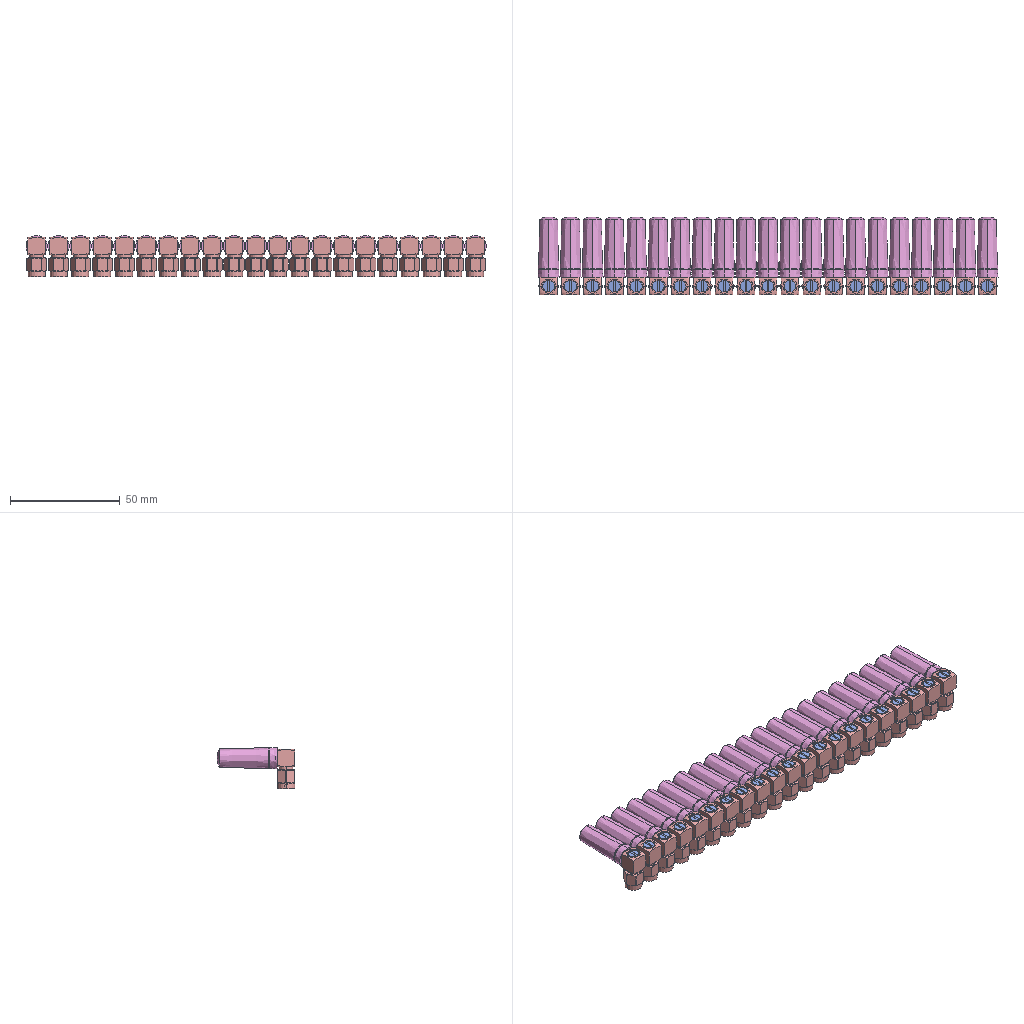Assembly | SolidWorks | 5 different items | 105 placed | box 210 x 36 x 19 mm
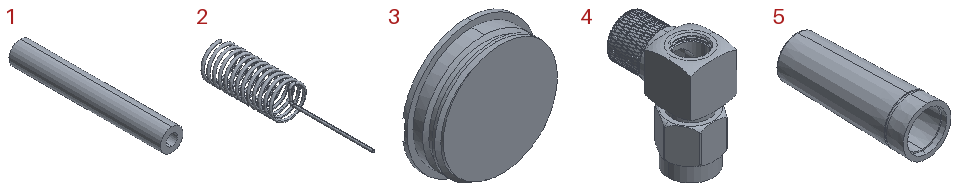Parts list (item | quantity | size | volume | features):
1 | x21 | 2 x 13.4 x 2 mm | 31.573 mm3 | features Extrusion 1
2 | x21 | 6.5 x 30.75 x 6.5 mm | 51.975 mm3 | features 3DProfileFeature 2, Helix 1, Sweep 1
3 | x21 | 5.4 x 1.3 x 5.4 mm | 23.765 mm3 | features ICE 3, Extrusion 1, Helix 1, SweepCut 1
4 | x21 | 9.176 x 15.05 x 17.9 mm | 892.261 mm3 | features ICE 11, Helix 3, SweepCut 3, RevCut 2, Chamfer 1, CirPattern 1, Extrusion 1, Fillet 1, MirrorPattern 1, Revolution 1
5 | x21 | 9.8 x 27.5 x 9.8 mm | 723.478 mm3 | features Revolution 1
Mates (type | each side: item.copy, entity, surface, feature):
Coordinate | 4.1 select_type:25 | assembly select_type:11
Coincident | 4.1 face plane Boss-Extrude1 | 3.1 face plane Boss-Extrude1
Parallel | 3.1 plane | assembly plane
Concentric | 4.1 edge | 3.1 edge
Tangent | 4.1 face cylinder Revolve1 | 2.1 face plane Sweep1
Concentric | 4.1 face cylinder Boss-Extrude2 | 2.1 face cylinder Sweep1
Concentric | 4.1 face cylinder Boss-Extrude6 | 5.1 face cone Revolve1
Coincident | 4.1 face plane Boss-Extrude1 | 5.1 face plane Revolve1
Concentric | 2.1 face cylinder Sweep1 | 1.1 face cylinder Boss-Extrude1
Coincident | 2.1 edge | 1.1 face plane Boss-Extrude1